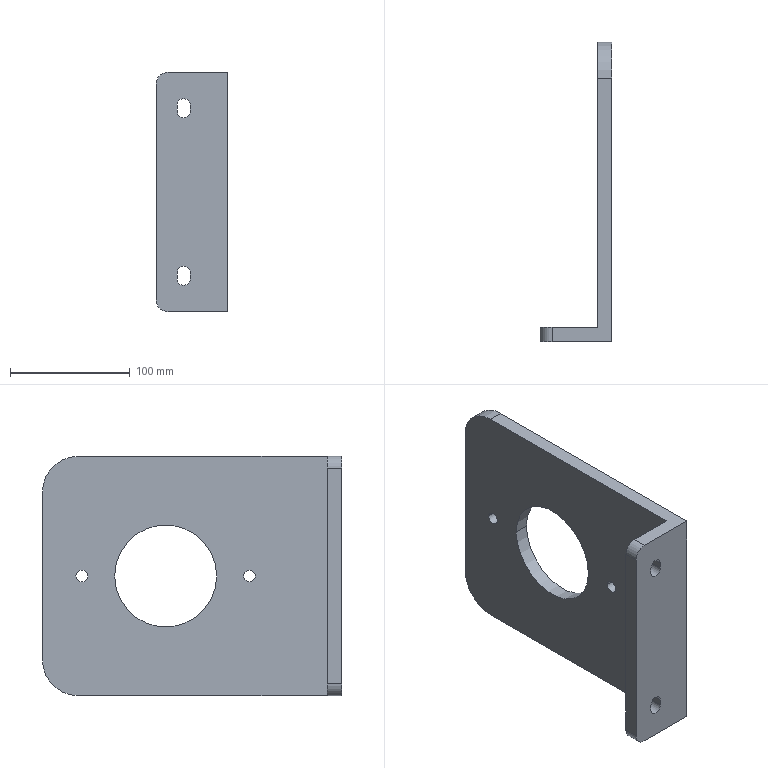Part | SolidWorks | features Fillet 2, ICE 2, Extrusion 1 | 1 solid | 26 faces | box 60 x 250 x 200 mm | volume 636149 mm3 | cylinder 14 | plane 12 | commonest cylinder face diameters 10 x4 11 x4 20 x2 60 x2 85.2 x2
STEP:
#1=CARTESIAN_POINT('',(0.,82.,0.));
#2=VERTEX_POINT('',#1);
#3=CARTESIAN_POINT('',(0.,72.,0.));
#4=VERTEX_POINT('',#3);
#5=CARTESIAN_POINT('',(0.,77.,0.));
#6=DIRECTION('',(-1.,0.,0.));
#7=DIRECTION('',(0.,1.,0.));
#8=AXIS2_PLACEMENT_3D('',#5,#6,#7);
#9=CIRCLE('',#8,5.);
#10=EDGE_CURVE('',#2,#4,#9,.T.);
#11=ORIENTED_EDGE('',*,*,#10,.F.);
#12=CARTESIAN_POINT('',(-12.,82.,0.));
#13=VERTEX_POINT('',#12);
#14=CARTESIAN_POINT('',(0.,82.,0.));
#15=DIRECTION('',(-1.,0.,0.));
#16=VECTOR('',#15,1000.);
#17=LINE('',#14,#16);
#18=EDGE_CURVE('',#2,#13,#17,.T.);
#19=ORIENTED_EDGE('',*,*,#18,.T.);
#20=CARTESIAN_POINT('',(-12.,72.,0.));
#21=VERTEX_POINT('',#20);
#22=CARTESIAN_POINT('',(-12.,77.,0.));
#23=DIRECTION('',(-1.,0.,0.));
#24=DIRECTION('',(0.,1.,0.));
#25=AXIS2_PLACEMENT_3D('',#22,#23,#24);
#26=CIRCLE('',#25,5.);
#27=EDGE_CURVE('',#13,#21,#26,.T.);
#28=ORIENTED_EDGE('',*,*,#27,.T.);
#29=CARTESIAN_POINT('',(0.,72.,0.));
#30=DIRECTION('',(-1.,0.,0.));
#31=VECTOR('',#30,1000.);
#32=LINE('',#29,#31);
#33=EDGE_CURVE('',#4,#21,#32,.T.);
#34=ORIENTED_EDGE('',*,*,#33,.F.);
#35=EDGE_LOOP('',(#11,#19,#28,#34));
#36=FACE_OUTER_BOUND('',#35,.T.);
#37=CARTESIAN_POINT('',(0.,77.,0.));
#38=DIRECTION('',(-1.,0.,0.));
#39=DIRECTION('',(0.,-1.,0.));
#40=AXIS2_PLACEMENT_3D('',#37,#38,#39);
#41=CYLINDRICAL_SURFACE('',#40,5.);
#42=ADVANCED_FACE('',(#36),#41,.F.);
#43=CARTESIAN_POINT('',(0.,222.,0.));
#44=VERTEX_POINT('',#43);
#45=CARTESIAN_POINT('',(0.,212.,0.));
#46=VERTEX_POINT('',#45);
#47=CARTESIAN_POINT('',(0.,217.,0.));
#48=DIRECTION('',(-1.,0.,0.));
#49=DIRECTION('',(0.,-1.,0.));
#50=AXIS2_PLACEMENT_3D('',#47,#48,#49);
#51=CIRCLE('',#50,5.);
#52=EDGE_CURVE('',#44,#46,#51,.T.);
#53=ORIENTED_EDGE('',*,*,#52,.F.);
#54=CARTESIAN_POINT('',(-12.,222.,0.));
#55=VERTEX_POINT('',#54);
#56=CARTESIAN_POINT('',(0.,222.,0.));
#57=DIRECTION('',(-1.,0.,0.));
#58=VECTOR('',#57,1000.);
#59=LINE('',#56,#58);
#60=EDGE_CURVE('',#44,#55,#59,.T.);
#61=ORIENTED_EDGE('',*,*,#60,.T.);
#62=CARTESIAN_POINT('',(-12.,212.,0.));
#63=VERTEX_POINT('',#62);
#64=CARTESIAN_POINT('',(-12.,217.,0.));
#65=DIRECTION('',(-1.,0.,0.));
#66=DIRECTION('',(0.,-1.,0.));
#67=AXIS2_PLACEMENT_3D('',#64,#65,#66);
#68=CIRCLE('',#67,5.);
#69=EDGE_CURVE('',#55,#63,#68,.T.);
#70=ORIENTED_EDGE('',*,*,#69,.T.);
#71=CARTESIAN_POINT('',(0.,212.,0.));
#72=DIRECTION('',(-1.,0.,0.));
#73=VECTOR('',#72,1000.);
#74=LINE('',#71,#73);
#75=EDGE_CURVE('',#46,#63,#74,.T.);
#76=ORIENTED_EDGE('',*,*,#75,.F.);
#77=EDGE_LOOP('',(#53,#61,#70,#76));
#78=FACE_OUTER_BOUND('',#77,.T.);
#79=CARTESIAN_POINT('',(0.,217.,0.));
#80=DIRECTION('',(-1.,0.,0.));
#81=DIRECTION('',(0.,-1.,0.));
#82=AXIS2_PLACEMENT_3D('',#79,#80,#81);
#83=CYLINDRICAL_SURFACE('',#82,5.);
#84=ADVANCED_FACE('',(#78),#83,.F.);
#85=CARTESIAN_POINT('',(0.,189.6,0.));
#86=VERTEX_POINT('',#85);
#87=CARTESIAN_POINT('',(0.,104.4,0.));
#88=VERTEX_POINT('',#87);
#89=CARTESIAN_POINT('',(0.,147.,0.));
#90=DIRECTION('',(-1.,0.,0.));
#91=DIRECTION('',(0.,-1.,0.));
#92=AXIS2_PLACEMENT_3D('',#89,#90,#91);
#93=CIRCLE('',#92,42.6);
#94=EDGE_CURVE('',#86,#88,#93,.T.);
#95=ORIENTED_EDGE('',*,*,#94,.F.);
#96=CARTESIAN_POINT('',(-12.,189.6,0.));
#97=VERTEX_POINT('',#96);
#98=CARTESIAN_POINT('',(0.,189.6,0.));
#99=DIRECTION('',(-1.,0.,0.));
#100=VECTOR('',#99,1000.);
#101=LINE('',#98,#100);
#102=EDGE_CURVE('',#86,#97,#101,.T.);
#103=ORIENTED_EDGE('',*,*,#102,.T.);
#104=CARTESIAN_POINT('',(-12.,104.4,0.));
#105=VERTEX_POINT('',#104);
#106=CARTESIAN_POINT('',(-12.,147.,0.));
#107=DIRECTION('',(-1.,0.,0.));
#108=DIRECTION('',(0.,-1.,0.));
#109=AXIS2_PLACEMENT_3D('',#106,#107,#108);
#110=CIRCLE('',#109,42.6);
#111=EDGE_CURVE('',#97,#105,#110,.T.);
#112=ORIENTED_EDGE('',*,*,#111,.T.);
#113=CARTESIAN_POINT('',(0.,104.4,0.));
#114=DIRECTION('',(-1.,0.,0.));
#115=VECTOR('',#114,1000.);
#116=LINE('',#113,#115);
#117=EDGE_CURVE('',#88,#105,#116,.T.);
#118=ORIENTED_EDGE('',*,*,#117,.F.);
#119=EDGE_LOOP('',(#95,#103,#112,#118));
#120=FACE_OUTER_BOUND('',#119,.T.);
#121=CARTESIAN_POINT('',(0.,147.,0.));
#122=DIRECTION('',(-1.,0.,0.));
#123=DIRECTION('',(0.,-1.,0.));
#124=AXIS2_PLACEMENT_3D('',#121,#122,#123);
#125=CYLINDRICAL_SURFACE('',#124,42.6);
#126=ADVANCED_FACE('',(#120),#125,.F.);
#127=CARTESIAN_POINT('',(-60.,12.,90.));
#128=VERTEX_POINT('',#127);
#129=CARTESIAN_POINT('',(-60.,12.,-90.));
#130=VERTEX_POINT('',#129);
#131=CARTESIAN_POINT('',(-60.,12.,100.));
#132=DIRECTION('',(0.,0.,-1.));
#133=VECTOR('',#132,1000.);
#134=LINE('',#131,#133);
#135=EDGE_CURVE('',#128,#130,#134,.T.);
#136=ORIENTED_EDGE('',*,*,#135,.T.);
#137=CARTESIAN_POINT('',(-60.,0.,-90.));
#138=VERTEX_POINT('',#137);
#139=CARTESIAN_POINT('',(-60.,12.,-90.));
#140=DIRECTION('',(0.,-1.,0.));
#141=VECTOR('',#140,1000.);
#142=LINE('',#139,#141);
#143=EDGE_CURVE('',#130,#138,#142,.T.);
#144=ORIENTED_EDGE('',*,*,#143,.T.);
#145=CARTESIAN_POINT('',(-60.,0.,90.));
#146=VERTEX_POINT('',#145);
#147=CARTESIAN_POINT('',(-60.,0.,100.));
#148=DIRECTION('',(0.,0.,-1.));
#149=VECTOR('',#148,1000.);
#150=LINE('',#147,#149);
#151=EDGE_CURVE('',#146,#138,#150,.T.);
#152=ORIENTED_EDGE('',*,*,#151,.F.);
#153=CARTESIAN_POINT('',(-60.,12.,90.));
#154=DIRECTION('',(0.,1.,0.));
#155=VECTOR('',#154,1000.);
#156=LINE('',#153,#155);
#157=EDGE_CURVE('',#146,#128,#156,.T.);
#158=ORIENTED_EDGE('',*,*,#157,.T.);
#159=EDGE_LOOP('',(#136,#144,#152,#158));
#160=FACE_OUTER_BOUND('',#159,.T.);
#161=CARTESIAN_POINT('',(-60.,12.,100.));
#162=DIRECTION('',(1.,0.,0.));
#163=DIRECTION('',(0.,0.,-1.));
#164=AXIS2_PLACEMENT_3D('',#161,#162,#163);
#165=PLANE('',#164);
#166=ADVANCED_FACE('',(#160),#165,.F.);
#167=CARTESIAN_POINT('',(-42.5,0.,-72.5));
#168=VERTEX_POINT('',#167);
#169=CARTESIAN_POINT('',(-42.5,0.,-67.5));
#170=VERTEX_POINT('',#169);
#171=CARTESIAN_POINT('',(-42.5,0.,-67.5));
#172=DIRECTION('',(0.,0.,1.));
#173=VECTOR('',#172,1000.);
#174=LINE('',#171,#173);
#175=EDGE_CURVE('',#168,#170,#174,.T.);
#176=ORIENTED_EDGE('',*,*,#175,.T.);
#177=CARTESIAN_POINT('',(-31.5,0.,-67.5));
#178=VERTEX_POINT('',#177);
#179=CARTESIAN_POINT('',(-37.,0.,-67.5));
#180=DIRECTION('',(0.,1.,0.));
#181=DIRECTION('',(-1.,0.,0.));
#182=AXIS2_PLACEMENT_3D('',#179,#180,#181);
#183=CIRCLE('',#182,5.5);
#184=EDGE_CURVE('',#170,#178,#183,.T.);
#185=ORIENTED_EDGE('',*,*,#184,.T.);
#186=CARTESIAN_POINT('',(-31.5,0.,-72.5));
#187=VERTEX_POINT('',#186);
#188=CARTESIAN_POINT('',(-31.5,0.,-67.5));
#189=DIRECTION('',(0.,0.,-1.));
#190=VECTOR('',#189,1000.);
#191=LINE('',#188,#190);
#192=EDGE_CURVE('',#178,#187,#191,.T.);
#193=ORIENTED_EDGE('',*,*,#192,.T.);
#194=CARTESIAN_POINT('',(-37.,0.,-72.5));
#195=DIRECTION('',(0.,1.,0.));
#196=DIRECTION('',(-1.,0.,0.));
#197=AXIS2_PLACEMENT_3D('',#194,#195,#196);
#198=CIRCLE('',#197,5.5);
#199=EDGE_CURVE('',#187,#168,#198,.T.);
#200=ORIENTED_EDGE('',*,*,#199,.T.);
#201=EDGE_LOOP('',(#176,#185,#193,#200));
#202=FACE_BOUND('',#201,.T.);
#203=CARTESIAN_POINT('',(-31.5,0.,72.5));
#204=VERTEX_POINT('',#203);
#205=CARTESIAN_POINT('',(-31.5,0.,67.5));
#206=VERTEX_POINT('',#205);
#207=CARTESIAN_POINT('',(-31.5,0.,67.5));
#208=DIRECTION('',(0.,0.,-1.));
#209=VECTOR('',#208,1000.);
#210=LINE('',#207,#209);
#211=EDGE_CURVE('',#204,#206,#210,.T.);
#212=ORIENTED_EDGE('',*,*,#211,.T.);
#213=CARTESIAN_POINT('',(-42.5,0.,67.5));
#214=VERTEX_POINT('',#213);
#215=CARTESIAN_POINT('',(-37.,0.,67.5));
#216=DIRECTION('',(0.,1.,0.));
#217=DIRECTION('',(1.,0.,0.));
#218=AXIS2_PLACEMENT_3D('',#215,#216,#217);
#219=CIRCLE('',#218,5.5);
#220=EDGE_CURVE('',#206,#214,#219,.T.);
#221=ORIENTED_EDGE('',*,*,#220,.T.);
#222=CARTESIAN_POINT('',(-42.5,0.,72.5));
#223=VERTEX_POINT('',#222);
#224=CARTESIAN_POINT('',(-42.5,0.,67.5));
#225=DIRECTION('',(0.,0.,1.));
#226=VECTOR('',#225,1000.);
#227=LINE('',#224,#226);
#228=EDGE_CURVE('',#214,#223,#227,.T.);
#229=ORIENTED_EDGE('',*,*,#228,.T.);
#230=CARTESIAN_POINT('',(-37.,0.,72.5));
#231=DIRECTION('',(0.,1.,0.));
#232=DIRECTION('',(1.,0.,0.));
#233=AXIS2_PLACEMENT_3D('',#230,#231,#232);
#234=CIRCLE('',#233,5.5);
#235=EDGE_CURVE('',#223,#204,#234,.T.);
#236=ORIENTED_EDGE('',*,*,#235,.T.);
#237=EDGE_LOOP('',(#212,#221,#229,#236));
#238=FACE_BOUND('',#237,.T.);
#239=ORIENTED_EDGE('',*,*,#151,.T.);
#240=CARTESIAN_POINT('',(-50.,0.,-100.));
#241=VERTEX_POINT('',#240);
#242=CARTESIAN_POINT('',(-50.,0.,-90.));
#243=DIRECTION('',(0.,-1.,0.));
#244=DIRECTION('',(0.,0.,1.));
#245=AXIS2_PLACEMENT_3D('',#242,#243,#244);
#246=CIRCLE('',#245,10.);
#247=EDGE_CURVE('',#138,#241,#246,.T.);
#248=ORIENTED_EDGE('',*,*,#247,.T.);
#249=CARTESIAN_POINT('',(0.,0.,-100.));
#250=VERTEX_POINT('',#249);
#251=CARTESIAN_POINT('',(-60.,0.,-100.));
#252=DIRECTION('',(1.,0.,0.));
#253=VECTOR('',#252,1000.);
#254=LINE('',#251,#253);
#255=EDGE_CURVE('',#241,#250,#254,.T.);
#256=ORIENTED_EDGE('',*,*,#255,.T.);
#257=CARTESIAN_POINT('',(0.,0.,100.));
#258=VERTEX_POINT('',#257);
#259=CARTESIAN_POINT('',(0.,0.,100.));
#260=DIRECTION('',(0.,0.,-1.));
#261=VECTOR('',#260,1000.);
#262=LINE('',#259,#261);
#263=EDGE_CURVE('',#258,#250,#262,.T.);
#264=ORIENTED_EDGE('',*,*,#263,.F.);
#265=CARTESIAN_POINT('',(-50.,0.,100.));
#266=VERTEX_POINT('',#265);
#267=CARTESIAN_POINT('',(-60.,0.,100.));
#268=DIRECTION('',(1.,0.,0.));
#269=VECTOR('',#268,1000.);
#270=LINE('',#267,#269);
#271=EDGE_CURVE('',#266,#258,#270,.T.);
#272=ORIENTED_EDGE('',*,*,#271,.F.);
#273=CARTESIAN_POINT('',(-50.,0.,90.));
#274=DIRECTION('',(0.,-1.,0.));
#275=DIRECTION('',(0.,0.,1.));
#276=AXIS2_PLACEMENT_3D('',#273,#274,#275);
#277=CIRCLE('',#276,10.);
#278=EDGE_CURVE('',#266,#146,#277,.T.);
#279=ORIENTED_EDGE('',*,*,#278,.T.);
#280=EDGE_LOOP('',(#239,#248,#256,#264,#272,#279));
#281=FACE_OUTER_BOUND('',#280,.T.);
#282=CARTESIAN_POINT('',(-60.,0.,100.));
#283=DIRECTION('',(0.,1.,0.));
#284=DIRECTION('',(0.,0.,1.));
#285=AXIS2_PLACEMENT_3D('',#282,#283,#284);
#286=PLANE('',#285);
#287=ADVANCED_FACE('',(#202,#238,#281),#286,.F.);
#288=CARTESIAN_POINT('',(0.,77.,0.));
#289=DIRECTION('',(-1.,0.,0.));
#290=DIRECTION('',(0.,1.,0.));
#291=AXIS2_PLACEMENT_3D('',#288,#289,#290);
#292=CIRCLE('',#291,5.);
#293=EDGE_CURVE('',#4,#2,#292,.T.);
#294=ORIENTED_EDGE('',*,*,#293,.T.);
#295=ORIENTED_EDGE('',*,*,#10,.T.);
#296=EDGE_LOOP('',(#294,#295));
#297=FACE_BOUND('',#296,.T.);
#298=CARTESIAN_POINT('',(0.,217.,0.));
#299=DIRECTION('',(-1.,0.,0.));
#300=DIRECTION('',(0.,-1.,0.));
#301=AXIS2_PLACEMENT_3D('',#298,#299,#300);
#302=CIRCLE('',#301,5.);
#303=EDGE_CURVE('',#46,#44,#302,.T.);
#304=ORIENTED_EDGE('',*,*,#303,.T.);
#305=ORIENTED_EDGE('',*,*,#52,.T.);
#306=EDGE_LOOP('',(#304,#305));
#307=FACE_BOUND('',#306,.T.);
#308=CARTESIAN_POINT('',(0.,147.,0.));
#309=DIRECTION('',(-1.,0.,0.));
#310=DIRECTION('',(0.,-1.,0.));
#311=AXIS2_PLACEMENT_3D('',#308,#309,#310);
#312=CIRCLE('',#311,42.6);
#313=EDGE_CURVE('',#88,#86,#312,.T.);
#314=ORIENTED_EDGE('',*,*,#313,.T.);
#315=ORIENTED_EDGE('',*,*,#94,.T.);
#316=EDGE_LOOP('',(#314,#315));
#317=FACE_BOUND('',#316,.T.);
#318=CARTESIAN_POINT('',(0.,220.,-100.));
#319=VERTEX_POINT('',#318);
#320=CARTESIAN_POINT('',(0.,0.,-100.));
#321=DIRECTION('',(0.,1.,0.));
#322=VECTOR('',#321,1000.);
#323=LINE('',#320,#322);
#324=EDGE_CURVE('',#250,#319,#323,.T.);
#325=ORIENTED_EDGE('',*,*,#324,.T.);
#326=CARTESIAN_POINT('',(0.,250.,-70.));
#327=VERTEX_POINT('',#326);
#328=CARTESIAN_POINT('',(0.,220.,-70.));
#329=DIRECTION('',(1.,0.,0.));
#330=DIRECTION('',(0.,-1.,0.));
#331=AXIS2_PLACEMENT_3D('',#328,#329,#330);
#332=CIRCLE('',#331,30.);
#333=EDGE_CURVE('',#319,#327,#332,.T.);
#334=ORIENTED_EDGE('',*,*,#333,.T.);
#335=CARTESIAN_POINT('',(0.,250.,70.));
#336=VERTEX_POINT('',#335);
#337=CARTESIAN_POINT('',(0.,250.,100.));
#338=DIRECTION('',(0.,0.,-1.));
#339=VECTOR('',#338,1000.);
#340=LINE('',#337,#339);
#341=EDGE_CURVE('',#336,#327,#340,.T.);
#342=ORIENTED_EDGE('',*,*,#341,.F.);
#343=CARTESIAN_POINT('',(0.,220.,100.));
#344=VERTEX_POINT('',#343);
#345=CARTESIAN_POINT('',(0.,220.,70.));
#346=DIRECTION('',(1.,0.,0.));
#347=DIRECTION('',(0.,-1.,0.));
#348=AXIS2_PLACEMENT_3D('',#345,#346,#347);
#349=CIRCLE('',#348,30.);
#350=EDGE_CURVE('',#336,#344,#349,.T.);
#351=ORIENTED_EDGE('',*,*,#350,.T.);
#352=CARTESIAN_POINT('',(0.,0.,100.));
#353=DIRECTION('',(0.,1.,0.));
#354=VECTOR('',#353,1000.);
#355=LINE('',#352,#354);
#356=EDGE_CURVE('',#258,#344,#355,.T.);
#357=ORIENTED_EDGE('',*,*,#356,.F.);
#358=ORIENTED_EDGE('',*,*,#263,.T.);
#359=EDGE_LOOP('',(#325,#334,#342,#351,#357,#358));
#360=FACE_OUTER_BOUND('',#359,.T.);
#361=CARTESIAN_POINT('',(0.,0.,100.));
#362=DIRECTION('',(-1.,0.,0.));
#363=DIRECTION('',(0.,-1.,0.));
#364=AXIS2_PLACEMENT_3D('',#361,#362,#363);
#365=PLANE('',#364);
#366=ADVANCED_FACE('',(#297,#307,#317,#360),#365,.F.);
#367=ORIENTED_EDGE('',*,*,#341,.T.);
#368=CARTESIAN_POINT('',(-12.,250.,-70.));
#369=VERTEX_POINT('',#368);
#370=CARTESIAN_POINT('',(0.,250.,-70.));
#371=DIRECTION('',(-1.,0.,0.));
#372=VECTOR('',#371,1000.);
#373=LINE('',#370,#372);
#374=EDGE_CURVE('',#327,#369,#373,.T.);
#375=ORIENTED_EDGE('',*,*,#374,.T.);
#376=CARTESIAN_POINT('',(-12.,250.,70.));
#377=VERTEX_POINT('',#376);
#378=CARTESIAN_POINT('',(-12.,250.,100.));
#379=DIRECTION('',(0.,0.,-1.));
#380=VECTOR('',#379,1000.);
#381=LINE('',#378,#380);
#382=EDGE_CURVE('',#377,#369,#381,.T.);
#383=ORIENTED_EDGE('',*,*,#382,.F.);
#384=CARTESIAN_POINT('',(0.,250.,70.));
#385=DIRECTION('',(1.,0.,0.));
#386=VECTOR('',#385,1000.);
#387=LINE('',#384,#386);
#388=EDGE_CURVE('',#377,#336,#387,.T.);
#389=ORIENTED_EDGE('',*,*,#388,.T.);
#390=EDGE_LOOP('',(#367,#375,#383,#389));
#391=FACE_OUTER_BOUND('',#390,.T.);
#392=CARTESIAN_POINT('',(0.,250.,100.));
#393=DIRECTION('',(0.,-1.,0.));
#394=DIRECTION('',(0.,0.,-1.));
#395=AXIS2_PLACEMENT_3D('',#392,#393,#394);
#396=PLANE('',#395);
#397=ADVANCED_FACE('',(#391),#396,.F.);
#398=CARTESIAN_POINT('',(-12.,77.,0.));
#399=DIRECTION('',(-1.,0.,0.));
#400=DIRECTION('',(0.,1.,0.));
#401=AXIS2_PLACEMENT_3D('',#398,#399,#400);
#402=CIRCLE('',#401,5.);
#403=EDGE_CURVE('',#21,#13,#402,.T.);
#404=ORIENTED_EDGE('',*,*,#403,.F.);
#405=ORIENTED_EDGE('',*,*,#27,.F.);
#406=EDGE_LOOP('',(#404,#405));
#407=FACE_BOUND('',#406,.T.);
#408=CARTESIAN_POINT('',(-12.,217.,0.));
#409=DIRECTION('',(-1.,0.,0.));
#410=DIRECTION('',(0.,-1.,0.));
#411=AXIS2_PLACEMENT_3D('',#408,#409,#410);
#412=CIRCLE('',#411,5.);
#413=EDGE_CURVE('',#63,#55,#412,.T.);
#414=ORIENTED_EDGE('',*,*,#413,.F.);
#415=ORIENTED_EDGE('',*,*,#69,.F.);
#416=EDGE_LOOP('',(#414,#415));
#417=FACE_BOUND('',#416,.T.);
#418=CARTESIAN_POINT('',(-12.,147.,0.));
#419=DIRECTION('',(-1.,0.,0.));
#420=DIRECTION('',(0.,-1.,0.));
#421=AXIS2_PLACEMENT_3D('',#418,#419,#420);
#422=CIRCLE('',#421,42.6);
#423=EDGE_CURVE('',#105,#97,#422,.T.);
#424=ORIENTED_EDGE('',*,*,#423,.F.);
#425=ORIENTED_EDGE('',*,*,#111,.F.);
#426=EDGE_LOOP('',(#424,#425));
#427=FACE_BOUND('',#426,.T.);
#428=ORIENTED_EDGE('',*,*,#382,.T.);
#429=CARTESIAN_POINT('',(-12.,220.,-100.));
#430=VERTEX_POINT('',#429);
#431=CARTESIAN_POINT('',(-12.,220.,-70.));
#432=DIRECTION('',(-1.,0.,0.));
#433=DIRECTION('',(0.,1.,0.));
#434=AXIS2_PLACEMENT_3D('',#431,#432,#433);
#435=CIRCLE('',#434,30.);
#436=EDGE_CURVE('',#369,#430,#435,.T.);
#437=ORIENTED_EDGE('',*,*,#436,.T.);
#438=CARTESIAN_POINT('',(-12.,12.,-100.));
#439=VERTEX_POINT('',#438);
#440=CARTESIAN_POINT('',(-12.,250.,-100.));
#441=DIRECTION('',(0.,-1.,0.));
#442=VECTOR('',#441,1000.);
#443=LINE('',#440,#442);
#444=EDGE_CURVE('',#430,#439,#443,.T.);
#445=ORIENTED_EDGE('',*,*,#444,.T.);
#446=CARTESIAN_POINT('',(-12.,12.,100.));
#447=VERTEX_POINT('',#446);
#448=CARTESIAN_POINT('',(-12.,12.,100.));
#449=DIRECTION('',(0.,0.,-1.));
#450=VECTOR('',#449,1000.);
#451=LINE('',#448,#450);
#452=EDGE_CURVE('',#447,#439,#451,.T.);
#453=ORIENTED_EDGE('',*,*,#452,.F.);
#454=CARTESIAN_POINT('',(-12.,220.,100.));
#455=VERTEX_POINT('',#454);
#456=CARTESIAN_POINT('',(-12.,250.,100.));
#457=DIRECTION('',(0.,-1.,0.));
#458=VECTOR('',#457,1000.);
#459=LINE('',#456,#458);
#460=EDGE_CURVE('',#455,#447,#459,.T.);
#461=ORIENTED_EDGE('',*,*,#460,.F.);
#462=CARTESIAN_POINT('',(-12.,220.,70.));
#463=DIRECTION('',(-1.,0.,0.));
#464=DIRECTION('',(0.,1.,0.));
#465=AXIS2_PLACEMENT_3D('',#462,#463,#464);
#466=CIRCLE('',#465,30.);
#467=EDGE_CURVE('',#455,#377,#466,.T.);
#468=ORIENTED_EDGE('',*,*,#467,.T.);
#469=EDGE_LOOP('',(#428,#437,#445,#453,#461,#468));
#470=FACE_OUTER_BOUND('',#469,.T.);
#471=CARTESIAN_POINT('',(-12.,250.,100.));
#472=DIRECTION('',(1.,0.,0.));
#473=DIRECTION('',(0.,1.,0.));
#474=AXIS2_PLACEMENT_3D('',#471,#472,#473);
#475=PLANE('',#474);
#476=ADVANCED_FACE('',(#407,#417,#427,#470),#475,.F.);
#477=CARTESIAN_POINT('',(-31.5,12.,-67.5));
#478=VERTEX_POINT('',#477);
#479=CARTESIAN_POINT('',(-31.5,12.,-72.5));
#480=VERTEX_POINT('',#479);
#481=CARTESIAN_POINT('',(-31.5,12.,-67.5));
#482=DIRECTION('',(0.,0.,-1.));
#483=VECTOR('',#482,1000.);
#484=LINE('',#481,#483);
#485=EDGE_CURVE('',#478,#480,#484,.T.);
#486=ORIENTED_EDGE('',*,*,#485,.F.);
#487=CARTESIAN_POINT('',(-42.5,12.,-67.5));
#488=VERTEX_POINT('',#487);
#489=CARTESIAN_POINT('',(-37.,12.,-67.5));
#490=DIRECTION('',(0.,1.,0.));
#491=DIRECTION('',(-1.,0.,0.));
#492=AXIS2_PLACEMENT_3D('',#489,#490,#491);
#493=CIRCLE('',#492,5.5);
#494=EDGE_CURVE('',#488,#478,#493,.T.);
#495=ORIENTED_EDGE('',*,*,#494,.F.);
#496=CARTESIAN_POINT('',(-42.5,12.,-72.5));
#497=VERTEX_POINT('',#496);
#498=CARTESIAN_POINT('',(-42.5,12.,-67.5));
#499=DIRECTION('',(0.,0.,1.));
#500=VECTOR('',#499,1000.);
#501=LINE('',#498,#500);
#502=EDGE_CURVE('',#497,#488,#501,.T.);
#503=ORIENTED_EDGE('',*,*,#502,.F.);
#504=CARTESIAN_POINT('',(-37.,12.,-72.5));
#505=DIRECTION('',(0.,1.,0.));
#506=DIRECTION('',(-1.,0.,0.));
#507=AXIS2_PLACEMENT_3D('',#504,#505,#506);
#508=CIRCLE('',#507,5.5);
#509=EDGE_CURVE('',#480,#497,#508,.T.);
#510=ORIENTED_EDGE('',*,*,#509,.F.);
#511=EDGE_LOOP('',(#486,#495,#503,#510));
#512=FACE_BOUND('',#511,.T.);
#513=CARTESIAN_POINT('',(-42.5,12.,67.5));
#514=VERTEX_POINT('',#513);
#515=CARTESIAN_POINT('',(-42.5,12.,72.5));
#516=VERTEX_POINT('',#515);
#517=CARTESIAN_POINT('',(-42.5,12.,67.5));
#518=DIRECTION('',(0.,0.,1.));
#519=VECTOR('',#518,1000.);
#520=LINE('',#517,#519);
#521=EDGE_CURVE('',#514,#516,#520,.T.);
#522=ORIENTED_EDGE('',*,*,#521,.F.);
#523=CARTESIAN_POINT('',(-31.5,12.,67.5));
#524=VERTEX_POINT('',#523);
#525=CARTESIAN_POINT('',(-37.,12.,67.5));
#526=DIRECTION('',(0.,1.,0.));
#527=DIRECTION('',(1.,0.,0.));
#528=AXIS2_PLACEMENT_3D('',#525,#526,#527);
#529=CIRCLE('',#528,5.5);
#530=EDGE_CURVE('',#524,#514,#529,.T.);
#531=ORIENTED_EDGE('',*,*,#530,.F.);
#532=CARTESIAN_POINT('',(-31.5,12.,72.5));
#533=VERTEX_POINT('',#532);
#534=CARTESIAN_POINT('',(-31.5,12.,67.5));
#535=DIRECTION('',(0.,0.,-1.));
#536=VECTOR('',#535,1000.);
#537=LINE('',#534,#536);
#538=EDGE_CURVE('',#533,#524,#537,.T.);
#539=ORIENTED_EDGE('',*,*,#538,.F.);
#540=CARTESIAN_POINT('',(-37.,12.,72.5));
#541=DIRECTION('',(0.,1.,0.));
#542=DIRECTION('',(1.,0.,0.));
#543=AXIS2_PLACEMENT_3D('',#540,#541,#542);
#544=CIRCLE('',#543,5.5);
#545=EDGE_CURVE('',#516,#533,#544,.T.);
#546=ORIENTED_EDGE('',*,*,#545,.F.);
#547=EDGE_LOOP('',(#522,#531,#539,#546));
#548=FACE_BOUND('',#547,.T.);
#549=CARTESIAN_POINT('',(-50.,12.,-100.));
#550=VERTEX_POINT('',#549);
#551=CARTESIAN_POINT('',(-12.,12.,-100.));
#552=DIRECTION('',(-1.,0.,0.));
#553=VECTOR('',#552,1000.);
#554=LINE('',#551,#553);
#555=EDGE_CURVE('',#439,#550,#554,.T.);
#556=ORIENTED_EDGE('',*,*,#555,.T.);
#557=CARTESIAN_POINT('',(-50.,12.,-90.));
#558=DIRECTION('',(0.,1.,0.));
#559=DIRECTION('',(1.,0.,0.));
#560=AXIS2_PLACEMENT_3D('',#557,#558,#559);
#561=CIRCLE('',#560,10.);
#562=EDGE_CURVE('',#550,#130,#561,.T.);
#563=ORIENTED_EDGE('',*,*,#562,.T.);
#564=ORIENTED_EDGE('',*,*,#135,.F.);
#565=CARTESIAN_POINT('',(-50.,12.,100.));
#566=VERTEX_POINT('',#565);
#567=CARTESIAN_POINT('',(-50.,12.,90.));
#568=DIRECTION('',(0.,1.,0.));
#569=DIRECTION('',(1.,0.,0.));
#570=AXIS2_PLACEMENT_3D('',#567,#568,#569);
#571=CIRCLE('',#570,10.);
#572=EDGE_CURVE('',#128,#566,#571,.T.);
#573=ORIENTED_EDGE('',*,*,#572,.T.);
#574=CARTESIAN_POINT('',(-12.,12.,100.));
#575=DIRECTION('',(-1.,0.,0.));
#576=VECTOR('',#575,1000.);
#577=LINE('',#574,#576);
#578=EDGE_CURVE('',#447,#566,#577,.T.);
#579=ORIENTED_EDGE('',*,*,#578,.F.);
#580=ORIENTED_EDGE('',*,*,#452,.T.);
#581=EDGE_LOOP('',(#556,#563,#564,#573,#579,#580));
#582=FACE_OUTER_BOUND('',#581,.T.);
#583=CARTESIAN_POINT('',(-12.,12.,100.));
#584=DIRECTION('',(0.,-1.,0.));
#585=DIRECTION('',(1.,0.,0.));
#586=AXIS2_PLACEMENT_3D('',#583,#584,#585);
#587=PLANE('',#586);
#588=ADVANCED_FACE('',(#512,#548,#582),#587,.F.);
#589=ORIENTED_EDGE('',*,*,#578,.T.);
#590=CARTESIAN_POINT('',(-50.,0.,100.));
#591=DIRECTION('',(0.,-1.,0.));
#592=VECTOR('',#591,1000.);
#593=LINE('',#590,#592);
#594=EDGE_CURVE('',#566,#266,#593,.T.);
#595=ORIENTED_EDGE('',*,*,#594,.T.);
#596=ORIENTED_EDGE('',*,*,#271,.T.);
#597=ORIENTED_EDGE('',*,*,#356,.T.);
#598=CARTESIAN_POINT('',(-12.,220.,100.));
#599=DIRECTION('',(-1.,0.,0.));
#600=VECTOR('',#599,1000.);
#601=LINE('',#598,#600);
#602=EDGE_CURVE('',#344,#455,#601,.T.);
#603=ORIENTED_EDGE('',*,*,#602,.T.);
#604=ORIENTED_EDGE('',*,*,#460,.T.);
#605=EDGE_LOOP('',(#589,#595,#596,#597,#603,#604));
#606=FACE_OUTER_BOUND('',#605,.T.);
#607=CARTESIAN_POINT('',(0.,0.,100.));
#608=DIRECTION('',(0.,0.,1.));
#609=DIRECTION('',(1.,0.,0.));
#610=AXIS2_PLACEMENT_3D('',#607,#608,#609);
#611=PLANE('',#610);
#612=ADVANCED_FACE('',(#606),#611,.T.);
#613=ORIENTED_EDGE('',*,*,#255,.F.);
#614=CARTESIAN_POINT('',(-50.,0.,-100.));
#615=DIRECTION('',(0.,1.,0.));
#616=VECTOR('',#615,1000.);
#617=LINE('',#614,#616);
#618=EDGE_CURVE('',#241,#550,#617,.T.);
#619=ORIENTED_EDGE('',*,*,#618,.T.);
#620=ORIENTED_EDGE('',*,*,#555,.F.);
#621=ORIENTED_EDGE('',*,*,#444,.F.);
#622=CARTESIAN_POINT('',(0.,220.,-100.));
#623=DIRECTION('',(1.,0.,0.));
#624=VECTOR('',#623,1000.);
#625=LINE('',#622,#624);
#626=EDGE_CURVE('',#430,#319,#625,.T.);
#627=ORIENTED_EDGE('',*,*,#626,.T.);
#628=ORIENTED_EDGE('',*,*,#324,.F.);
#629=EDGE_LOOP('',(#613,#619,#620,#621,#627,#628));
#630=FACE_OUTER_BOUND('',#629,.T.);
#631=CARTESIAN_POINT('',(0.,0.,-100.));
#632=DIRECTION('',(0.,0.,1.));
#633=DIRECTION('',(1.,0.,0.));
#634=AXIS2_PLACEMENT_3D('',#631,#632,#633);
#635=PLANE('',#634);
#636=ADVANCED_FACE('',(#630),#635,.F.);
#637=ORIENTED_EDGE('',*,*,#530,.T.);
#638=CARTESIAN_POINT('',(-42.5,0.,67.5));
#639=DIRECTION('',(0.,1.,0.));
#640=VECTOR('',#639,1000.);
#641=LINE('',#638,#640);
#642=EDGE_CURVE('',#214,#514,#641,.T.);
#643=ORIENTED_EDGE('',*,*,#642,.F.);
#644=ORIENTED_EDGE('',*,*,#220,.F.);
#645=CARTESIAN_POINT('',(-31.5,0.,67.5));
#646=DIRECTION('',(0.,1.,0.));
#647=VECTOR('',#646,1000.);
#648=LINE('',#645,#647);
#649=EDGE_CURVE('',#206,#524,#648,.T.);
#650=ORIENTED_EDGE('',*,*,#649,.T.);
#651=EDGE_LOOP('',(#637,#643,#644,#650));
#652=FACE_OUTER_BOUND('',#651,.T.);
#653=CARTESIAN_POINT('',(-37.,0.,67.5));
#654=DIRECTION('',(0.,1.,0.));
#655=DIRECTION('',(-1.,0.,0.));
#656=AXIS2_PLACEMENT_3D('',#653,#654,#655);
#657=CYLINDRICAL_SURFACE('',#656,5.5);
#658=ADVANCED_FACE('',(#652),#657,.F.);
#659=ORIENTED_EDGE('',*,*,#538,.T.);
#660=ORIENTED_EDGE('',*,*,#649,.F.);
#661=ORIENTED_EDGE('',*,*,#211,.F.);
#662=CARTESIAN_POINT('',(-31.5,0.,72.5));
#663=DIRECTION('',(0.,1.,0.));
#664=VECTOR('',#663,1000.);
#665=LINE('',#662,#664);
#666=EDGE_CURVE('',#204,#533,#665,.T.);
#667=ORIENTED_EDGE('',*,*,#666,.T.);
#668=EDGE_LOOP('',(#659,#660,#661,#667));
#669=FACE_OUTER_BOUND('',#668,.T.);
#670=CARTESIAN_POINT('',(-31.5,0.,67.5));
#671=DIRECTION('',(1.,0.,0.));
#672=DIRECTION('',(0.,1.,0.));
#673=AXIS2_PLACEMENT_3D('',#670,#671,#672);
#674=PLANE('',#673);
#675=ADVANCED_FACE('',(#669),#674,.F.);
#676=ORIENTED_EDGE('',*,*,#545,.T.);
#677=ORIENTED_EDGE('',*,*,#666,.F.);
#678=ORIENTED_EDGE('',*,*,#235,.F.);
#679=CARTESIAN_POINT('',(-42.5,0.,72.5));
#680=DIRECTION('',(0.,1.,0.));
#681=VECTOR('',#680,1000.);
#682=LINE('',#679,#681);
#683=EDGE_CURVE('',#223,#516,#682,.T.);
#684=ORIENTED_EDGE('',*,*,#683,.T.);
#685=EDGE_LOOP('',(#676,#677,#678,#684));
#686=FACE_OUTER_BOUND('',#685,.T.);
#687=CARTESIAN_POINT('',(-37.,0.,72.5));
#688=DIRECTION('',(0.,1.,0.));
#689=DIRECTION('',(-1.,0.,0.));
#690=AXIS2_PLACEMENT_3D('',#687,#688,#689);
#691=CYLINDRICAL_SURFACE('',#690,5.5);
#692=ADVANCED_FACE('',(#686),#691,.F.);
#693=ORIENTED_EDGE('',*,*,#521,.T.);
#694=ORIENTED_EDGE('',*,*,#683,.F.);
#695=ORIENTED_EDGE('',*,*,#228,.F.);
#696=ORIENTED_EDGE('',*,*,#642,.T.);
#697=EDGE_LOOP('',(#693,#694,#695,#696));
#698=FACE_OUTER_BOUND('',#697,.T.);
#699=CARTESIAN_POINT('',(-42.5,0.,67.5));
#700=DIRECTION('',(-1.,0.,0.));
#701=DIRECTION('',(0.,-1.,0.));
#702=AXIS2_PLACEMENT_3D('',#699,#700,#701);
#703=PLANE('',#702);
#704=ADVANCED_FACE('',(#698),#703,.F.);
#705=ORIENTED_EDGE('',*,*,#494,.T.);
#706=CARTESIAN_POINT('',(-31.5,0.,-67.5));
#707=DIRECTION('',(0.,1.,0.));
#708=VECTOR('',#707,1000.);
#709=LINE('',#706,#708);
#710=EDGE_CURVE('',#178,#478,#709,.T.);
#711=ORIENTED_EDGE('',*,*,#710,.F.);
#712=ORIENTED_EDGE('',*,*,#184,.F.);
#713=CARTESIAN_POINT('',(-42.5,0.,-67.5));
#714=DIRECTION('',(0.,1.,0.));
#715=VECTOR('',#714,1000.);
#716=LINE('',#713,#715);
#717=EDGE_CURVE('',#170,#488,#716,.T.);
#718=ORIENTED_EDGE('',*,*,#717,.T.);
#719=EDGE_LOOP('',(#705,#711,#712,#718));
#720=FACE_OUTER_BOUND('',#719,.T.);
#721=CARTESIAN_POINT('',(-37.,0.,-67.5));
#722=DIRECTION('',(0.,1.,0.));
#723=DIRECTION('',(-1.,0.,0.));
#724=AXIS2_PLACEMENT_3D('',#721,#722,#723);
#725=CYLINDRICAL_SURFACE('',#724,5.5);
#726=ADVANCED_FACE('',(#720),#725,.F.);
#727=ORIENTED_EDGE('',*,*,#502,.T.);
#728=ORIENTED_EDGE('',*,*,#717,.F.);
#729=ORIENTED_EDGE('',*,*,#175,.F.);
#730=CARTESIAN_POINT('',(-42.5,0.,-72.5));
#731=DIRECTION('',(0.,1.,0.));
#732=VECTOR('',#731,1000.);
#733=LINE('',#730,#732);
#734=EDGE_CURVE('',#168,#497,#733,.T.);
#735=ORIENTED_EDGE('',*,*,#734,.T.);
#736=EDGE_LOOP('',(#727,#728,#729,#735));
#737=FACE_OUTER_BOUND('',#736,.T.);
#738=CARTESIAN_POINT('',(-42.5,0.,-67.5));
#739=DIRECTION('',(-1.,0.,0.));
#740=DIRECTION('',(0.,-1.,0.));
#741=AXIS2_PLACEMENT_3D('',#738,#739,#740);
#742=PLANE('',#741);
#743=ADVANCED_FACE('',(#737),#742,.F.);
#744=ORIENTED_EDGE('',*,*,#509,.T.);
#745=ORIENTED_EDGE('',*,*,#734,.F.);
#746=ORIENTED_EDGE('',*,*,#199,.F.);
#747=CARTESIAN_POINT('',(-31.5,0.,-72.5));
#748=DIRECTION('',(0.,1.,0.));
#749=VECTOR('',#748,1000.);
#750=LINE('',#747,#749);
#751=EDGE_CURVE('',#187,#480,#750,.T.);
#752=ORIENTED_EDGE('',*,*,#751,.T.);
#753=EDGE_LOOP('',(#744,#745,#746,#752));
#754=FACE_OUTER_BOUND('',#753,.T.);
#755=CARTESIAN_POINT('',(-37.,0.,-72.5));
#756=DIRECTION('',(0.,1.,0.));
#757=DIRECTION('',(-1.,0.,0.));
#758=AXIS2_PLACEMENT_3D('',#755,#756,#757);
#759=CYLINDRICAL_SURFACE('',#758,5.5);
#760=ADVANCED_FACE('',(#754),#759,.F.);
#761=ORIENTED_EDGE('',*,*,#485,.T.);
#762=ORIENTED_EDGE('',*,*,#751,.F.);
#763=ORIENTED_EDGE('',*,*,#192,.F.);
#764=ORIENTED_EDGE('',*,*,#710,.T.);
#765=EDGE_LOOP('',(#761,#762,#763,#764));
#766=FACE_OUTER_BOUND('',#765,.T.);
#767=CARTESIAN_POINT('',(-31.5,0.,-67.5));
#768=DIRECTION('',(1.,0.,0.));
#769=DIRECTION('',(0.,1.,0.));
#770=AXIS2_PLACEMENT_3D('',#767,#768,#769);
#771=PLANE('',#770);
#772=ADVANCED_FACE('',(#766),#771,.F.);
#773=ORIENTED_EDGE('',*,*,#102,.F.);
#774=ORIENTED_EDGE('',*,*,#313,.F.);
#775=ORIENTED_EDGE('',*,*,#117,.T.);
#776=ORIENTED_EDGE('',*,*,#423,.T.);
#777=EDGE_LOOP('',(#773,#774,#775,#776));
#778=FACE_OUTER_BOUND('',#777,.T.);
#779=CARTESIAN_POINT('',(0.,147.,0.));
#780=DIRECTION('',(-1.,0.,0.));
#781=DIRECTION('',(0.,-1.,0.));
#782=AXIS2_PLACEMENT_3D('',#779,#780,#781);
#783=CYLINDRICAL_SURFACE('',#782,42.6);
#784=ADVANCED_FACE('',(#778),#783,.F.);
#785=ORIENTED_EDGE('',*,*,#60,.F.);
#786=ORIENTED_EDGE('',*,*,#303,.F.);
#787=ORIENTED_EDGE('',*,*,#75,.T.);
#788=ORIENTED_EDGE('',*,*,#413,.T.);
#789=EDGE_LOOP('',(#785,#786,#787,#788));
#790=FACE_OUTER_BOUND('',#789,.T.);
#791=CARTESIAN_POINT('',(0.,217.,0.));
#792=DIRECTION('',(-1.,0.,0.));
#793=DIRECTION('',(0.,-1.,0.));
#794=AXIS2_PLACEMENT_3D('',#791,#792,#793);
#795=CYLINDRICAL_SURFACE('',#794,5.);
#796=ADVANCED_FACE('',(#790),#795,.F.);
#797=ORIENTED_EDGE('',*,*,#18,.F.);
#798=ORIENTED_EDGE('',*,*,#293,.F.);
#799=ORIENTED_EDGE('',*,*,#33,.T.);
#800=ORIENTED_EDGE('',*,*,#403,.T.);
#801=EDGE_LOOP('',(#797,#798,#799,#800));
#802=FACE_OUTER_BOUND('',#801,.T.);
#803=CARTESIAN_POINT('',(0.,77.,0.));
#804=DIRECTION('',(-1.,0.,0.));
#805=DIRECTION('',(0.,-1.,0.));
#806=AXIS2_PLACEMENT_3D('',#803,#804,#805);
#807=CYLINDRICAL_SURFACE('',#806,5.);
#808=ADVANCED_FACE('',(#802),#807,.F.);
#809=ORIENTED_EDGE('',*,*,#333,.F.);
#810=ORIENTED_EDGE('',*,*,#626,.F.);
#811=ORIENTED_EDGE('',*,*,#436,.F.);
#812=ORIENTED_EDGE('',*,*,#374,.F.);
#813=EDGE_LOOP('',(#809,#810,#811,#812));
#814=FACE_OUTER_BOUND('',#813,.T.);
#815=CARTESIAN_POINT('',(0.,220.,-70.));
#816=DIRECTION('',(-1.,0.,0.));
#817=DIRECTION('',(0.,0.,1.));
#818=AXIS2_PLACEMENT_3D('',#815,#816,#817);
#819=CYLINDRICAL_SURFACE('',#818,30.);
#820=ADVANCED_FACE('',(#814),#819,.T.);
#821=ORIENTED_EDGE('',*,*,#350,.F.);
#822=ORIENTED_EDGE('',*,*,#388,.F.);
#823=ORIENTED_EDGE('',*,*,#467,.F.);
#824=ORIENTED_EDGE('',*,*,#602,.F.);
#825=EDGE_LOOP('',(#821,#822,#823,#824));
#826=FACE_OUTER_BOUND('',#825,.T.);
#827=CARTESIAN_POINT('',(0.,220.,70.));
#828=DIRECTION('',(1.,0.,0.));
#829=DIRECTION('',(0.,0.,-1.));
#830=AXIS2_PLACEMENT_3D('',#827,#828,#829);
#831=CYLINDRICAL_SURFACE('',#830,30.);
#832=ADVANCED_FACE('',(#826),#831,.T.);
#833=ORIENTED_EDGE('',*,*,#562,.F.);
#834=ORIENTED_EDGE('',*,*,#618,.F.);
#835=ORIENTED_EDGE('',*,*,#247,.F.);
#836=ORIENTED_EDGE('',*,*,#143,.F.);
#837=EDGE_LOOP('',(#833,#834,#835,#836));
#838=FACE_OUTER_BOUND('',#837,.T.);
#839=CARTESIAN_POINT('',(-50.,12.,-90.));
#840=DIRECTION('',(0.,-1.,0.));
#841=DIRECTION('',(0.,0.,-1.));
#842=AXIS2_PLACEMENT_3D('',#839,#840,#841);
#843=CYLINDRICAL_SURFACE('',#842,10.);
#844=ADVANCED_FACE('',(#838),#843,.T.);
#845=ORIENTED_EDGE('',*,*,#572,.F.);
#846=ORIENTED_EDGE('',*,*,#157,.F.);
#847=ORIENTED_EDGE('',*,*,#278,.F.);
#848=ORIENTED_EDGE('',*,*,#594,.F.);
#849=EDGE_LOOP('',(#845,#846,#847,#848));
#850=FACE_OUTER_BOUND('',#849,.T.);
#851=CARTESIAN_POINT('',(-50.,0.,90.));
#852=DIRECTION('',(0.,1.,0.));
#853=DIRECTION('',(0.,0.,1.));
#854=AXIS2_PLACEMENT_3D('',#851,#852,#853);
#855=CYLINDRICAL_SURFACE('',#854,10.);
#856=ADVANCED_FACE('',(#850),#855,.T.);
#857=CLOSED_SHELL('',(#42,#84,#126,#166,#287,#366,#397,#476,#588,#612,#636,#658,#675,#692,#704,#726,#743,#760,#772,#784,#796,#808,#820,#832,#844,#856));
#858=MANIFOLD_SOLID_BREP('',#857);
#859=CARTESIAN_POINT('',(0.,0.,0.));
#860=DIRECTION('',(0.,0.,1.));
#861=DIRECTION('',(1.,0.,0.));
#862=AXIS2_PLACEMENT_3D('',#859,#860,#861);
#863=(LENGTH_UNIT()NAMED_UNIT(*)SI_UNIT(.MILLI.,.METRE.));
#864=UNCERTAINTY_MEASURE_WITH_UNIT(LENGTH_MEASURE(0.00001),#863,'','');
#865=(NAMED_UNIT(*)PLANE_ANGLE_UNIT()SI_UNIT($,.RADIAN.));
#866=(NAMED_UNIT(*)SI_UNIT($,.STERADIAN.)SOLID_ANGLE_UNIT());
#867=(GEOMETRIC_REPRESENTATION_CONTEXT(3)GLOBAL_UNCERTAINTY_ASSIGNED_CONTEXT((#864))GLOBAL_UNIT_ASSIGNED_CONTEXT((#863,#865,#866))REPRESENTATION_CONTEXT('',''));
#868=ADVANCED_BREP_SHAPE_REPRESENTATION('',(#858,#862),#867);